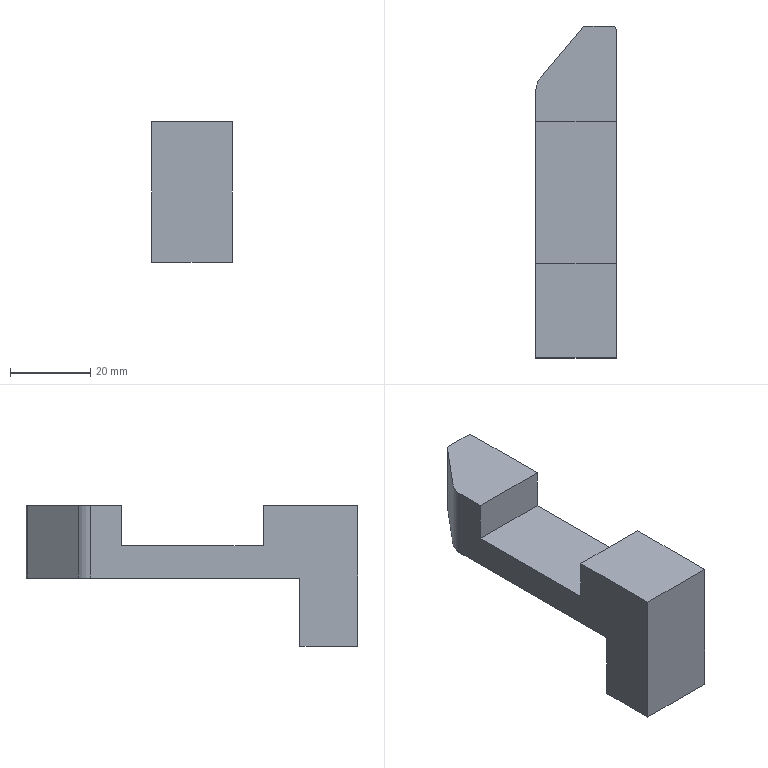Part | STEP file | lll_id4714_x_t | 1 solid | 16 faces | box 20 x 82.5 x 35 mm | volume 25991 mm3 | plane 13 | cylinder 3 | commonest cylinder face diameters 2 x2 10 x1
STEP:
#1=CARTESIAN_POINT('',(775.37,-406.832,0.));
#2=VERTEX_POINT('',#1);
#3=CARTESIAN_POINT('',(795.37,-406.832,0.));
#4=VERTEX_POINT('',#3);
#5=CARTESIAN_POINT('',(754.393,-406.832,0.));
#6=DIRECTION('',(1.,0.,0.));
#7=VECTOR('',#6,1.);
#8=LINE('',#5,#7);
#9=EDGE_CURVE('',#2,#4,#8,.T.);
#10=ORIENTED_EDGE('',*,*,#9,.F.);
#11=CARTESIAN_POINT('',(775.37,-354.871,0.));
#12=VERTEX_POINT('',#11);
#13=CARTESIAN_POINT('',(775.37,-399.832,0.));
#14=DIRECTION('',(0.,1.,0.));
#15=VECTOR('',#14,1.);
#16=LINE('',#13,#15);
#17=EDGE_CURVE('',#2,#12,#16,.T.);
#18=ORIENTED_EDGE('',*,*,#17,.T.);
#19=CARTESIAN_POINT('',(776.54,-351.657,0.));
#20=VERTEX_POINT('',#19);
#21=CARTESIAN_POINT('',(780.37,-354.871,0.));
#22=DIRECTION('',(0.,0.,-1.));
#23=DIRECTION('',(1.,0.,0.));
#24=AXIS2_PLACEMENT_3D('',#21,#22,#23);
#25=CIRCLE('',#24,5.);
#26=EDGE_CURVE('',#12,#20,#25,.T.);
#27=ORIENTED_EDGE('',*,*,#26,.T.);
#28=CARTESIAN_POINT('',(787.071,-339.107,0.));
#29=VERTEX_POINT('',#28);
#30=CARTESIAN_POINT('',(776.54,-351.657,0.));
#31=DIRECTION('',(0.6428,0.766,0.));
#32=VECTOR('',#31,1.);
#33=LINE('',#30,#32);
#34=EDGE_CURVE('',#20,#29,#33,.T.);
#35=ORIENTED_EDGE('',*,*,#34,.T.);
#36=CARTESIAN_POINT('',(787.837,-338.75,0.));
#37=VERTEX_POINT('',#36);
#38=CARTESIAN_POINT('',(787.837,-339.75,0.));
#39=DIRECTION('',(0.,0.,-1.));
#40=DIRECTION('',(1.,0.,0.));
#41=AXIS2_PLACEMENT_3D('',#38,#39,#40);
#42=CIRCLE('',#41,1.);
#43=EDGE_CURVE('',#29,#37,#42,.T.);
#44=ORIENTED_EDGE('',*,*,#43,.T.);
#45=CARTESIAN_POINT('',(794.37,-338.75,0.));
#46=VERTEX_POINT('',#45);
#47=CARTESIAN_POINT('',(787.837,-338.75,0.));
#48=DIRECTION('',(1.,0.,0.));
#49=VECTOR('',#48,1.);
#50=LINE('',#47,#49);
#51=EDGE_CURVE('',#37,#46,#50,.T.);
#52=ORIENTED_EDGE('',*,*,#51,.T.);
#53=CARTESIAN_POINT('',(795.37,-339.75,0.));
#54=VERTEX_POINT('',#53);
#55=CARTESIAN_POINT('',(794.37,-339.75,0.));
#56=DIRECTION('',(0.,0.,-1.));
#57=DIRECTION('',(1.,0.,0.));
#58=AXIS2_PLACEMENT_3D('',#55,#56,#57);
#59=CIRCLE('',#58,1.);
#60=EDGE_CURVE('',#46,#54,#59,.T.);
#61=ORIENTED_EDGE('',*,*,#60,.T.);
#62=CARTESIAN_POINT('',(795.37,-339.75,0.));
#63=DIRECTION('',(0.,-1.,0.));
#64=VECTOR('',#63,1.);
#65=LINE('',#62,#64);
#66=EDGE_CURVE('',#54,#4,#65,.T.);
#67=ORIENTED_EDGE('',*,*,#66,.T.);
#68=EDGE_LOOP('',(#10,#18,#27,#35,#44,#52,#61,#67));
#69=FACE_OUTER_BOUND('',#68,.T.);
#70=CARTESIAN_POINT('',(754.393,99.43,0.));
#71=DIRECTION('',(0.,0.,1.));
#72=DIRECTION('',(-1.,0.,0.));
#73=AXIS2_PLACEMENT_3D('',#70,#71,#72);
#74=PLANE('',#73);
#75=ADVANCED_FACE('',(#69),#74,.F.);
#76=CARTESIAN_POINT('',(775.37,-421.25,18.));
#77=VERTEX_POINT('',#76);
#78=CARTESIAN_POINT('',(775.37,-421.25,-17.));
#79=VERTEX_POINT('',#78);
#80=CARTESIAN_POINT('',(775.37,-421.25,-2.));
#81=DIRECTION('',(0.,0.,-1.));
#82=VECTOR('',#81,1.);
#83=LINE('',#80,#82);
#84=EDGE_CURVE('',#77,#79,#83,.T.);
#85=ORIENTED_EDGE('',*,*,#84,.F.);
#86=CARTESIAN_POINT('',(775.37,-397.7,18.));
#87=VERTEX_POINT('',#86);
#88=CARTESIAN_POINT('',(775.37,-394.832,18.));
#89=DIRECTION('',(0.,1.,0.));
#90=VECTOR('',#89,1.);
#91=LINE('',#88,#90);
#92=EDGE_CURVE('',#77,#87,#91,.T.);
#93=ORIENTED_EDGE('',*,*,#92,.T.);
#94=CARTESIAN_POINT('',(775.37,-397.7,8.));
#95=VERTEX_POINT('',#94);
#96=CARTESIAN_POINT('',(775.37,-397.7,-2.));
#97=DIRECTION('',(0.,0.,1.));
#98=VECTOR('',#97,1.);
#99=LINE('',#96,#98);
#100=EDGE_CURVE('',#95,#87,#99,.T.);
#101=ORIENTED_EDGE('',*,*,#100,.F.);
#102=CARTESIAN_POINT('',(775.37,-362.421,8.));
#103=VERTEX_POINT('',#102);
#104=CARTESIAN_POINT('',(775.37,-379.291,8.));
#105=DIRECTION('',(0.,1.,0.));
#106=VECTOR('',#105,1.);
#107=LINE('',#104,#106);
#108=EDGE_CURVE('',#95,#103,#107,.T.);
#109=ORIENTED_EDGE('',*,*,#108,.T.);
#110=CARTESIAN_POINT('',(775.37,-362.421,18.));
#111=VERTEX_POINT('',#110);
#112=CARTESIAN_POINT('',(775.37,-362.421,-2.));
#113=DIRECTION('',(0.,0.,1.));
#114=VECTOR('',#113,1.);
#115=LINE('',#112,#114);
#116=EDGE_CURVE('',#103,#111,#115,.T.);
#117=ORIENTED_EDGE('',*,*,#116,.T.);
#118=CARTESIAN_POINT('',(775.37,-354.871,18.));
#119=VERTEX_POINT('',#118);
#120=CARTESIAN_POINT('',(775.37,-399.832,18.));
#121=DIRECTION('',(0.,1.,0.));
#122=VECTOR('',#121,1.);
#123=LINE('',#120,#122);
#124=EDGE_CURVE('',#111,#119,#123,.T.);
#125=ORIENTED_EDGE('',*,*,#124,.T.);
#126=CARTESIAN_POINT('',(775.37,-354.871,-2.));
#127=DIRECTION('',(0.,0.,1.));
#128=VECTOR('',#127,1.);
#129=LINE('',#126,#128);
#130=EDGE_CURVE('',#12,#119,#129,.T.);
#131=ORIENTED_EDGE('',*,*,#130,.F.);
#132=ORIENTED_EDGE('',*,*,#17,.F.);
#133=CARTESIAN_POINT('',(775.37,-406.832,-17.));
#134=VERTEX_POINT('',#133);
#135=CARTESIAN_POINT('',(775.37,-406.832,-2.));
#136=DIRECTION('',(0.,0.,1.));
#137=VECTOR('',#136,1.);
#138=LINE('',#135,#137);
#139=EDGE_CURVE('',#134,#2,#138,.T.);
#140=ORIENTED_EDGE('',*,*,#139,.F.);
#141=CARTESIAN_POINT('',(775.37,-399.832,-17.));
#142=DIRECTION('',(0.,-1.,0.));
#143=VECTOR('',#142,1.);
#144=LINE('',#141,#143);
#145=EDGE_CURVE('',#134,#79,#144,.T.);
#146=ORIENTED_EDGE('',*,*,#145,.T.);
#147=EDGE_LOOP('',(#85,#93,#101,#109,#117,#125,#131,#132,#140,#146));
#148=FACE_OUTER_BOUND('',#147,.T.);
#149=CARTESIAN_POINT('',(775.37,-399.832,-2.));
#150=DIRECTION('',(-1.,0.,0.));
#151=DIRECTION('',(0.,0.,1.));
#152=AXIS2_PLACEMENT_3D('',#149,#150,#151);
#153=PLANE('',#152);
#154=ADVANCED_FACE('',(#148),#153,.T.);
#155=ORIENTED_EDGE('',*,*,#130,.T.);
#156=CARTESIAN_POINT('',(776.54,-351.657,18.));
#157=VERTEX_POINT('',#156);
#158=CARTESIAN_POINT('',(780.37,-354.871,18.));
#159=DIRECTION('',(0.,0.,-1.));
#160=DIRECTION('',(-1.,0.,0.));
#161=AXIS2_PLACEMENT_3D('',#158,#159,#160);
#162=CIRCLE('',#161,5.);
#163=EDGE_CURVE('',#119,#157,#162,.T.);
#164=ORIENTED_EDGE('',*,*,#163,.T.);
#165=CARTESIAN_POINT('',(776.54,-351.657,-2.));
#166=DIRECTION('',(0.,0.,1.));
#167=VECTOR('',#166,1.);
#168=LINE('',#165,#167);
#169=EDGE_CURVE('',#20,#157,#168,.T.);
#170=ORIENTED_EDGE('',*,*,#169,.F.);
#171=ORIENTED_EDGE('',*,*,#26,.F.);
#172=EDGE_LOOP('',(#155,#164,#170,#171));
#173=FACE_OUTER_BOUND('',#172,.T.);
#174=CARTESIAN_POINT('',(780.37,-354.871,-2.));
#175=DIRECTION('',(0.,0.,1.));
#176=DIRECTION('',(1.,0.,0.));
#177=AXIS2_PLACEMENT_3D('',#174,#175,#176);
#178=CYLINDRICAL_SURFACE('',#177,5.);
#179=ADVANCED_FACE('',(#173),#178,.T.);
#180=ORIENTED_EDGE('',*,*,#169,.T.);
#181=CARTESIAN_POINT('',(787.071,-339.107,18.));
#182=VERTEX_POINT('',#181);
#183=CARTESIAN_POINT('',(776.54,-351.657,18.));
#184=DIRECTION('',(0.6428,0.766,0.));
#185=VECTOR('',#184,1.);
#186=LINE('',#183,#185);
#187=EDGE_CURVE('',#157,#182,#186,.T.);
#188=ORIENTED_EDGE('',*,*,#187,.T.);
#189=CARTESIAN_POINT('',(787.071,-339.107,-2.));
#190=DIRECTION('',(0.,0.,1.));
#191=VECTOR('',#190,1.);
#192=LINE('',#189,#191);
#193=EDGE_CURVE('',#29,#182,#192,.T.);
#194=ORIENTED_EDGE('',*,*,#193,.F.);
#195=ORIENTED_EDGE('',*,*,#34,.F.);
#196=EDGE_LOOP('',(#180,#188,#194,#195));
#197=FACE_OUTER_BOUND('',#196,.T.);
#198=CARTESIAN_POINT('',(776.54,-351.657,-2.));
#199=DIRECTION('',(-0.766,0.6428,0.));
#200=DIRECTION('',(-0.6428,-0.766,0.));
#201=AXIS2_PLACEMENT_3D('',#198,#199,#200);
#202=PLANE('',#201);
#203=ADVANCED_FACE('',(#197),#202,.T.);
#204=ORIENTED_EDGE('',*,*,#193,.T.);
#205=CARTESIAN_POINT('',(787.837,-338.75,18.));
#206=VERTEX_POINT('',#205);
#207=CARTESIAN_POINT('',(787.837,-339.75,18.));
#208=DIRECTION('',(0.,0.,-1.));
#209=DIRECTION('',(-1.,0.,0.));
#210=AXIS2_PLACEMENT_3D('',#207,#208,#209);
#211=CIRCLE('',#210,1.);
#212=EDGE_CURVE('',#182,#206,#211,.T.);
#213=ORIENTED_EDGE('',*,*,#212,.T.);
#214=CARTESIAN_POINT('',(787.837,-338.75,-2.));
#215=DIRECTION('',(0.,0.,1.));
#216=VECTOR('',#215,1.);
#217=LINE('',#214,#216);
#218=EDGE_CURVE('',#37,#206,#217,.T.);
#219=ORIENTED_EDGE('',*,*,#218,.F.);
#220=ORIENTED_EDGE('',*,*,#43,.F.);
#221=EDGE_LOOP('',(#204,#213,#219,#220));
#222=FACE_OUTER_BOUND('',#221,.T.);
#223=CARTESIAN_POINT('',(787.837,-339.75,-2.));
#224=DIRECTION('',(0.,0.,1.));
#225=DIRECTION('',(1.,0.,0.));
#226=AXIS2_PLACEMENT_3D('',#223,#224,#225);
#227=CYLINDRICAL_SURFACE('',#226,1.);
#228=ADVANCED_FACE('',(#222),#227,.T.);
#229=ORIENTED_EDGE('',*,*,#218,.T.);
#230=CARTESIAN_POINT('',(794.37,-338.75,18.));
#231=VERTEX_POINT('',#230);
#232=CARTESIAN_POINT('',(787.837,-338.75,18.));
#233=DIRECTION('',(1.,0.,0.));
#234=VECTOR('',#233,1.);
#235=LINE('',#232,#234);
#236=EDGE_CURVE('',#206,#231,#235,.T.);
#237=ORIENTED_EDGE('',*,*,#236,.T.);
#238=CARTESIAN_POINT('',(794.37,-338.75,-2.));
#239=DIRECTION('',(0.,0.,1.));
#240=VECTOR('',#239,1.);
#241=LINE('',#238,#240);
#242=EDGE_CURVE('',#46,#231,#241,.T.);
#243=ORIENTED_EDGE('',*,*,#242,.F.);
#244=ORIENTED_EDGE('',*,*,#51,.F.);
#245=EDGE_LOOP('',(#229,#237,#243,#244));
#246=FACE_OUTER_BOUND('',#245,.T.);
#247=CARTESIAN_POINT('',(787.837,-338.75,-2.));
#248=DIRECTION('',(0.,1.,0.));
#249=DIRECTION('',(-1.,0.,0.));
#250=AXIS2_PLACEMENT_3D('',#247,#248,#249);
#251=PLANE('',#250);
#252=ADVANCED_FACE('',(#246),#251,.T.);
#253=ORIENTED_EDGE('',*,*,#242,.T.);
#254=CARTESIAN_POINT('',(795.37,-339.75,18.));
#255=VERTEX_POINT('',#254);
#256=CARTESIAN_POINT('',(794.37,-339.75,18.));
#257=DIRECTION('',(0.,0.,-1.));
#258=DIRECTION('',(-1.,0.,0.));
#259=AXIS2_PLACEMENT_3D('',#256,#257,#258);
#260=CIRCLE('',#259,1.);
#261=EDGE_CURVE('',#231,#255,#260,.T.);
#262=ORIENTED_EDGE('',*,*,#261,.T.);
#263=CARTESIAN_POINT('',(795.37,-339.75,-2.));
#264=DIRECTION('',(0.,0.,1.));
#265=VECTOR('',#264,1.);
#266=LINE('',#263,#265);
#267=EDGE_CURVE('',#54,#255,#266,.T.);
#268=ORIENTED_EDGE('',*,*,#267,.F.);
#269=ORIENTED_EDGE('',*,*,#60,.F.);
#270=EDGE_LOOP('',(#253,#262,#268,#269));
#271=FACE_OUTER_BOUND('',#270,.T.);
#272=CARTESIAN_POINT('',(794.37,-339.75,-2.));
#273=DIRECTION('',(0.,0.,1.));
#274=DIRECTION('',(1.,0.,0.));
#275=AXIS2_PLACEMENT_3D('',#272,#273,#274);
#276=CYLINDRICAL_SURFACE('',#275,1.);
#277=ADVANCED_FACE('',(#271),#276,.T.);
#278=CARTESIAN_POINT('',(795.37,-421.25,18.));
#279=VERTEX_POINT('',#278);
#280=CARTESIAN_POINT('',(795.37,-421.25,-17.));
#281=VERTEX_POINT('',#280);
#282=CARTESIAN_POINT('',(795.37,-421.25,9.));
#283=DIRECTION('',(0.,0.,-1.));
#284=VECTOR('',#283,1.);
#285=LINE('',#282,#284);
#286=EDGE_CURVE('',#279,#281,#285,.T.);
#287=ORIENTED_EDGE('',*,*,#286,.T.);
#288=CARTESIAN_POINT('',(795.37,-406.832,-17.));
#289=VERTEX_POINT('',#288);
#290=CARTESIAN_POINT('',(795.37,-427.832,-17.));
#291=DIRECTION('',(0.,-1.,0.));
#292=VECTOR('',#291,1.);
#293=LINE('',#290,#292);
#294=EDGE_CURVE('',#289,#281,#293,.T.);
#295=ORIENTED_EDGE('',*,*,#294,.F.);
#296=CARTESIAN_POINT('',(795.37,-406.832,-2.));
#297=DIRECTION('',(0.,0.,1.));
#298=VECTOR('',#297,1.);
#299=LINE('',#296,#298);
#300=EDGE_CURVE('',#289,#4,#299,.T.);
#301=ORIENTED_EDGE('',*,*,#300,.T.);
#302=ORIENTED_EDGE('',*,*,#66,.F.);
#303=ORIENTED_EDGE('',*,*,#267,.T.);
#304=CARTESIAN_POINT('',(795.37,-362.421,18.));
#305=VERTEX_POINT('',#304);
#306=CARTESIAN_POINT('',(795.37,-339.75,18.));
#307=DIRECTION('',(0.,-1.,0.));
#308=VECTOR('',#307,1.);
#309=LINE('',#306,#308);
#310=EDGE_CURVE('',#255,#305,#309,.T.);
#311=ORIENTED_EDGE('',*,*,#310,.T.);
#312=CARTESIAN_POINT('',(795.37,-362.421,8.));
#313=VERTEX_POINT('',#312);
#314=CARTESIAN_POINT('',(795.37,-362.421,-2.));
#315=DIRECTION('',(0.,0.,-1.));
#316=VECTOR('',#315,1.);
#317=LINE('',#314,#316);
#318=EDGE_CURVE('',#305,#313,#317,.T.);
#319=ORIENTED_EDGE('',*,*,#318,.T.);
#320=CARTESIAN_POINT('',(795.37,-397.7,8.));
#321=VERTEX_POINT('',#320);
#322=CARTESIAN_POINT('',(795.37,-379.291,8.));
#323=DIRECTION('',(0.,-1.,0.));
#324=VECTOR('',#323,1.);
#325=LINE('',#322,#324);
#326=EDGE_CURVE('',#313,#321,#325,.T.);
#327=ORIENTED_EDGE('',*,*,#326,.T.);
#328=CARTESIAN_POINT('',(795.37,-397.7,18.));
#329=VERTEX_POINT('',#328);
#330=CARTESIAN_POINT('',(795.37,-397.7,-2.));
#331=DIRECTION('',(0.,0.,-1.));
#332=VECTOR('',#331,1.);
#333=LINE('',#330,#332);
#334=EDGE_CURVE('',#329,#321,#333,.T.);
#335=ORIENTED_EDGE('',*,*,#334,.F.);
#336=CARTESIAN_POINT('',(795.37,-334.75,18.));
#337=DIRECTION('',(0.,-1.,0.));
#338=VECTOR('',#337,1.);
#339=LINE('',#336,#338);
#340=EDGE_CURVE('',#329,#279,#339,.T.);
#341=ORIENTED_EDGE('',*,*,#340,.T.);
#342=EDGE_LOOP('',(#287,#295,#301,#302,#303,#311,#319,#327,#335,#341));
#343=FACE_OUTER_BOUND('',#342,.T.);
#344=CARTESIAN_POINT('',(795.37,-339.75,-2.));
#345=DIRECTION('',(1.,0.,0.));
#346=DIRECTION('',(0.,0.,-1.));
#347=AXIS2_PLACEMENT_3D('',#344,#345,#346);
#348=PLANE('',#347);
#349=ADVANCED_FACE('',(#343),#348,.T.);
#350=ORIENTED_EDGE('',*,*,#108,.F.);
#351=CARTESIAN_POINT('',(817.821,-397.7,8.));
#352=DIRECTION('',(1.,0.,0.));
#353=VECTOR('',#352,1.);
#354=LINE('',#351,#353);
#355=EDGE_CURVE('',#95,#321,#354,.T.);
#356=ORIENTED_EDGE('',*,*,#355,.T.);
#357=ORIENTED_EDGE('',*,*,#326,.F.);
#358=CARTESIAN_POINT('',(785.37,-362.421,8.));
#359=DIRECTION('',(-1.,0.,0.));
#360=VECTOR('',#359,1.);
#361=LINE('',#358,#360);
#362=EDGE_CURVE('',#313,#103,#361,.T.);
#363=ORIENTED_EDGE('',*,*,#362,.T.);
#364=EDGE_LOOP('',(#350,#356,#357,#363));
#365=FACE_OUTER_BOUND('',#364,.T.);
#366=CARTESIAN_POINT('',(785.37,-379.291,8.));
#367=DIRECTION('',(0.,0.,-1.));
#368=DIRECTION('',(-1.,0.,0.));
#369=AXIS2_PLACEMENT_3D('',#366,#367,#368);
#370=PLANE('',#369);
#371=ADVANCED_FACE('',(#365),#370,.F.);
#372=ORIENTED_EDGE('',*,*,#124,.F.);
#373=CARTESIAN_POINT('',(785.37,-362.421,18.));
#374=DIRECTION('',(-1.,0.,0.));
#375=VECTOR('',#374,1.);
#376=LINE('',#373,#375);
#377=EDGE_CURVE('',#305,#111,#376,.T.);
#378=ORIENTED_EDGE('',*,*,#377,.F.);
#379=ORIENTED_EDGE('',*,*,#310,.F.);
#380=ORIENTED_EDGE('',*,*,#261,.F.);
#381=ORIENTED_EDGE('',*,*,#236,.F.);
#382=ORIENTED_EDGE('',*,*,#212,.F.);
#383=ORIENTED_EDGE('',*,*,#187,.F.);
#384=ORIENTED_EDGE('',*,*,#163,.F.);
#385=EDGE_LOOP('',(#372,#378,#379,#380,#381,#382,#383,#384));
#386=FACE_OUTER_BOUND('',#385,.T.);
#387=CARTESIAN_POINT('',(780.37,-354.871,18.));
#388=DIRECTION('',(0.,0.,1.));
#389=DIRECTION('',(1.,0.,0.));
#390=AXIS2_PLACEMENT_3D('',#387,#388,#389);
#391=PLANE('',#390);
#392=ADVANCED_FACE('',(#386),#391,.T.);
#393=ORIENTED_EDGE('',*,*,#318,.F.);
#394=ORIENTED_EDGE('',*,*,#377,.T.);
#395=ORIENTED_EDGE('',*,*,#116,.F.);
#396=ORIENTED_EDGE('',*,*,#362,.F.);
#397=EDGE_LOOP('',(#393,#394,#395,#396));
#398=FACE_OUTER_BOUND('',#397,.T.);
#399=CARTESIAN_POINT('',(785.37,-362.421,12.));
#400=DIRECTION('',(0.,-1.,0.));
#401=DIRECTION('',(0.,0.,-1.));
#402=AXIS2_PLACEMENT_3D('',#399,#400,#401);
#403=PLANE('',#402);
#404=ADVANCED_FACE('',(#398),#403,.T.);
#405=CARTESIAN_POINT('',(780.37,-421.25,18.));
#406=DIRECTION('',(-1.,0.,0.));
#407=VECTOR('',#406,1.);
#408=LINE('',#405,#407);
#409=EDGE_CURVE('',#279,#77,#408,.T.);
#410=ORIENTED_EDGE('',*,*,#409,.F.);
#411=ORIENTED_EDGE('',*,*,#340,.F.);
#412=CARTESIAN_POINT('',(817.821,-397.7,18.));
#413=DIRECTION('',(-1.,0.,0.));
#414=VECTOR('',#413,1.);
#415=LINE('',#412,#414);
#416=EDGE_CURVE('',#329,#87,#415,.T.);
#417=ORIENTED_EDGE('',*,*,#416,.T.);
#418=ORIENTED_EDGE('',*,*,#92,.F.);
#419=EDGE_LOOP('',(#410,#411,#417,#418));
#420=FACE_OUTER_BOUND('',#419,.T.);
#421=CARTESIAN_POINT('',(780.37,-349.871,18.));
#422=DIRECTION('',(0.,0.,1.));
#423=DIRECTION('',(1.,0.,0.));
#424=AXIS2_PLACEMENT_3D('',#421,#422,#423);
#425=PLANE('',#424);
#426=ADVANCED_FACE('',(#420),#425,.T.);
#427=ORIENTED_EDGE('',*,*,#416,.F.);
#428=ORIENTED_EDGE('',*,*,#334,.T.);
#429=ORIENTED_EDGE('',*,*,#355,.F.);
#430=ORIENTED_EDGE('',*,*,#100,.T.);
#431=EDGE_LOOP('',(#427,#428,#429,#430));
#432=FACE_OUTER_BOUND('',#431,.T.);
#433=CARTESIAN_POINT('',(817.821,-397.7,11.5));
#434=DIRECTION('',(0.,1.,0.));
#435=DIRECTION('',(0.,0.,1.));
#436=AXIS2_PLACEMENT_3D('',#433,#434,#435);
#437=PLANE('',#436);
#438=ADVANCED_FACE('',(#432),#437,.T.);
#439=ORIENTED_EDGE('',*,*,#139,.T.);
#440=ORIENTED_EDGE('',*,*,#9,.T.);
#441=ORIENTED_EDGE('',*,*,#300,.F.);
#442=CARTESIAN_POINT('',(795.37,-406.832,-17.));
#443=DIRECTION('',(-1.,0.,0.));
#444=VECTOR('',#443,1.);
#445=LINE('',#442,#444);
#446=EDGE_CURVE('',#289,#134,#445,.T.);
#447=ORIENTED_EDGE('',*,*,#446,.T.);
#448=EDGE_LOOP('',(#439,#440,#441,#447));
#449=FACE_OUTER_BOUND('',#448,.T.);
#450=CARTESIAN_POINT('',(795.37,-406.832,-2.));
#451=DIRECTION('',(0.,-1.,0.));
#452=DIRECTION('',(0.,0.,1.));
#453=AXIS2_PLACEMENT_3D('',#450,#451,#452);
#454=PLANE('',#453);
#455=ADVANCED_FACE('',(#449),#454,.F.);
#456=CARTESIAN_POINT('',(795.37,-421.25,-17.));
#457=DIRECTION('',(1.,0.,0.));
#458=VECTOR('',#457,1.);
#459=LINE('',#456,#458);
#460=EDGE_CURVE('',#79,#281,#459,.T.);
#461=ORIENTED_EDGE('',*,*,#460,.F.);
#462=ORIENTED_EDGE('',*,*,#145,.F.);
#463=ORIENTED_EDGE('',*,*,#446,.F.);
#464=ORIENTED_EDGE('',*,*,#294,.T.);
#465=EDGE_LOOP('',(#461,#462,#463,#464));
#466=FACE_OUTER_BOUND('',#465,.T.);
#467=CARTESIAN_POINT('',(795.37,-427.832,-17.));
#468=DIRECTION('',(0.,0.,1.));
#469=DIRECTION('',(-1.,0.,0.));
#470=AXIS2_PLACEMENT_3D('',#467,#468,#469);
#471=PLANE('',#470);
#472=ADVANCED_FACE('',(#466),#471,.F.);
#473=ORIENTED_EDGE('',*,*,#409,.T.);
#474=ORIENTED_EDGE('',*,*,#84,.T.);
#475=ORIENTED_EDGE('',*,*,#460,.T.);
#476=ORIENTED_EDGE('',*,*,#286,.F.);
#477=EDGE_LOOP('',(#473,#474,#475,#476));
#478=FACE_OUTER_BOUND('',#477,.T.);
#479=CARTESIAN_POINT('',(791.104,-421.25,9.));
#480=DIRECTION('',(0.,1.,0.));
#481=DIRECTION('',(0.,0.,1.));
#482=AXIS2_PLACEMENT_3D('',#479,#480,#481);
#483=PLANE('',#482);
#484=ADVANCED_FACE('',(#478),#483,.F.);
#485=CLOSED_SHELL('',(#75,#154,#179,#203,#228,#252,#277,#349,#371,#392,#404,#426,#438,#455,#472,#484));
#486=MANIFOLD_SOLID_BREP('',#485);
#487=(LENGTH_UNIT()NAMED_UNIT(*)SI_UNIT(.MILLI.,.METRE.));
#488=UNCERTAINTY_MEASURE_WITH_UNIT(LENGTH_MEASURE(0.00002),#487,'','');
#489=(NAMED_UNIT(*)PLANE_ANGLE_UNIT()SI_UNIT($,.RADIAN.));
#490=PLANE_ANGLE_MEASURE_WITH_UNIT(PLANE_ANGLE_MEASURE(0.01745),#489);
#491=DIMENSIONAL_EXPONENTS(0.,0.,0.,0.,0.,0.,0.);
#492=(CONVERSION_BASED_UNIT('DEGREE',#490)NAMED_UNIT(#491)PLANE_ANGLE_UNIT());
#493=(NAMED_UNIT(*)SI_UNIT($,.STERADIAN.)SOLID_ANGLE_UNIT());
#494=(GEOMETRIC_REPRESENTATION_CONTEXT(3)GLOBAL_UNCERTAINTY_ASSIGNED_CONTEXT((#488))GLOBAL_UNIT_ASSIGNED_CONTEXT((#487,#492,#493))REPRESENTATION_CONTEXT('',''));
#495=ADVANCED_BREP_SHAPE_REPRESENTATION('',(#486),#494);